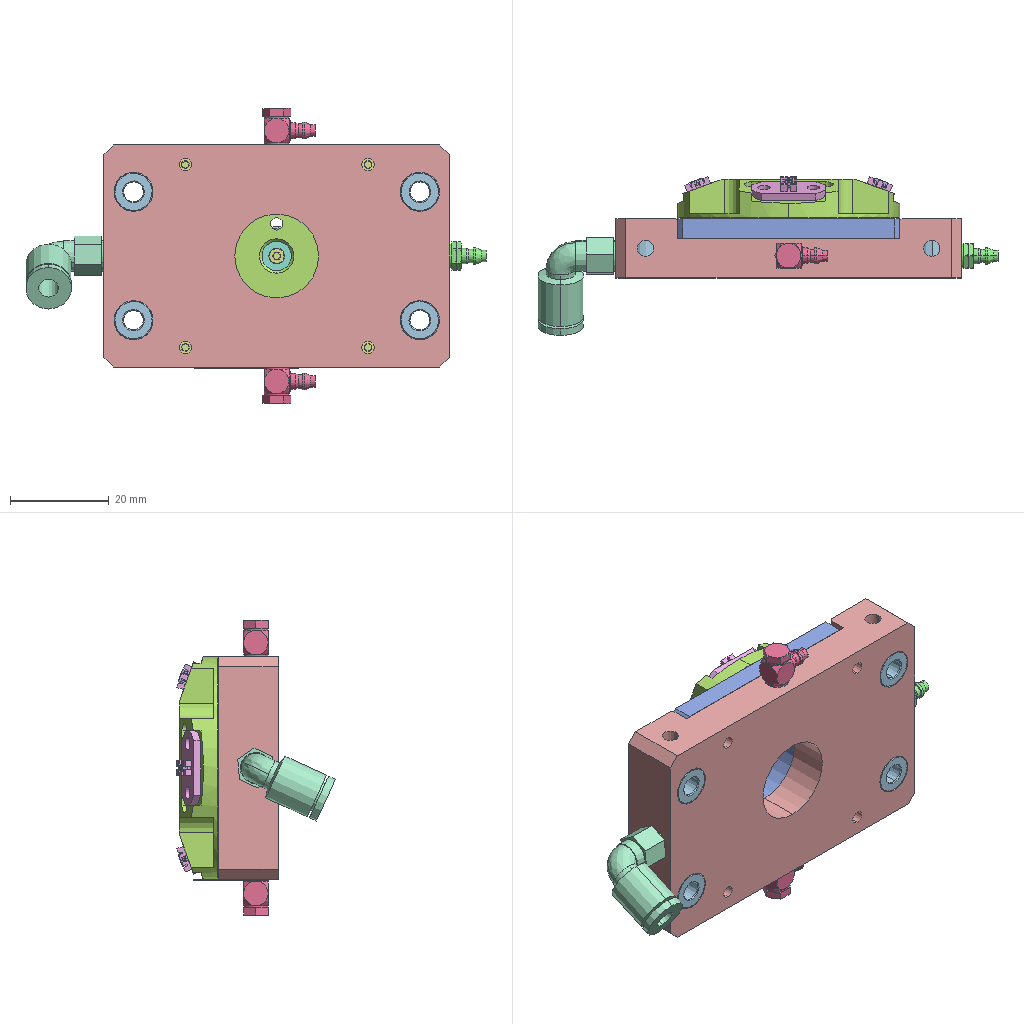Assembly | SolidWorks | 13 different items | 27 placed | box 93 x 32 x 60 mm
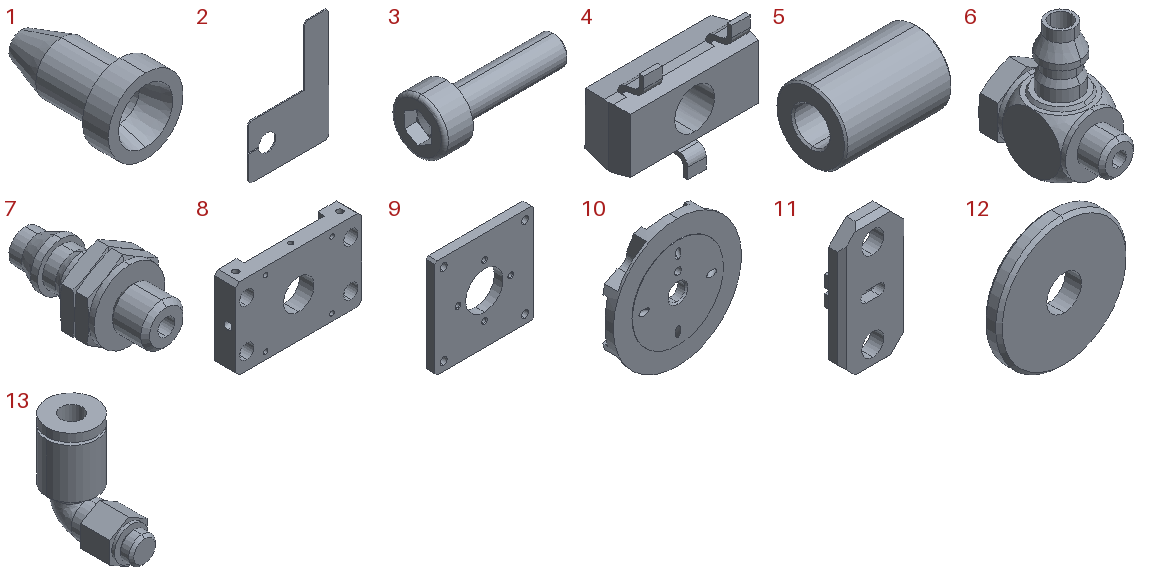Parts list (item | quantity | size | volume | features):
1 | x1 | 2.9 x 4.8 x 2.9 mm | 9.616 mm3 | features ICE 4, Chamfer 1, Extrusion 1, RevCut 1
2 | x1 | 15 x 0.2 x 21 mm | 38.09 mm3 | features ICE 3, Chamfer 1, FlatPattern 1, SMBaseFlange 1, SheetMetal 1
3 | x5 | 7.6 x 3 x 3 mm | 21.652 mm3 | features Fillet 2, RevCut 2, Boss 1, Chamfer 1, Cut 1, Extrusion 1, LPattern 1
4 | x4 | 2.908 x 1.057 x 2.408 mm | 2.992 mm3 | features ICE 6, Fillet 4, Extrusion 1, RefAxis 1
5 | x4 | 12 x 8 x 8 mm | 450.881 mm3 | features RefAxis 3, 3DProfileFeature 1, Chamfer 1, Revolution 1
6 | x2 | 5 x 9.5 x 10.687 mm | 200.167 mm3 | features BaseBody 1
7 | x1 | 5 x 10 x 5.774 mm | 89.646 mm3 | features BaseBody 1
8 | x1 | 70 x 12 x 45 mm | 24347 mm3 | features ICE 8, HoleWzd 6, 3DProfileFeature 4, Chamfer 2, CirPattern 1, Extrusion 1, MirrorPattern 1
9 | x1 | 45 x 4 x 45 mm | 6746 mm3 | features ICE 5, Chamfer 2, CirPattern 2, Cut 1, Extrusion 1, Fillet 1
10 | x1 | 45 x 8 x 45 mm | 6154 mm3 | features ICE 14, CirPattern 5, Chamfer 2, Extrusion 1, Fillet 1, HoleWzd 1
11 | x4 | 7 x 3 x 15 mm | 138.292 mm3 | features ICE 14, Chamfer 5, Extrusion 1
12 | x1 | 12 x 1.5 x 12 mm | 154.246 mm3 | features Chamfer 1, Extrusion 1
13 | x1 | 9.3 x 18.35 x 19.641 mm | 1123 mm3 | features BaseBody 1
Mates (type | each side: item.copy, entity, surface, feature):
Coincident | 8.1 face plane Cut-Extrude1 | 9.1 face plane Boss-Extrude1 | 2 times
Coincident | 8.1 face plane Boss-Extrude1 | 5.1 face plane Revolve1 | 2 times
Concentric | 8.1 face cylinder Cut-Extrude2 | 5.1 face cylinder Revolve1
Concentric | 8.1 face cylinder Cut-Extrude2 | 5.2 face cylinder Revolve1
Coincident | 8.1 face plane Boss-Extrude1 | 5.2 face plane Revolve1
Concentric | 8.1 face cylinder Cut-Extrude2 | 5.3 face cylinder Revolve1
Coincident | 8.1 face plane Boss-Extrude1 | 5.3 face plane Revolve1
Concentric | 8.1 face cylinder Cut-Extrude2 | 5.4 face cylinder Revolve1
Coincident | 8.1 face plane Boss-Extrude1 | 5.4 face plane Revolve1
Coincident | 10.1 face plane CirPattern2 | 11.1 face plane Boss-Extrude1 | 3 times
Coincident | 9.1 face plane Boss-Extrude1 | 10.1 face plane Boss-Extrude1
Concentric | 9.1 face cylinder Cut-Extrude1 | 10.1 face cylinder Boss-Extrude1
Coincident | 11.1 face plane Cut-Extrude1 | 4.1 face plane Boss-Extrude1
Concentric | 9.1 face cylinder Cut-Extrude6 | 3.1 face cylinder BaseBody
Concentric | 9.1 face cylinder CirPattern2 | 3.2 face cylinder BaseBody
Coincident | 9.1 face plane Cut-Extrude6 | 3.2 face plane BaseHead
Concentric | 9.1 face cylinder CirPattern2 | 3.3 face cylinder BaseBody
Coincident | 9.1 face plane Cut-Extrude6 | 3.3 face plane BaseHead
Concentric | 9.1 face cylinder Cut-Extrude4 | 3.4 face cylinder BaseBody
Coincident | 9.1 face plane Cut-Extrude6 | 3.4 face plane BaseHead
Coincident | 9.1 face plane Cut-Extrude6 | 3.1 face plane BaseHead
Coincident | 10.1 face plane Cut-Extrude4 | 12.1 face plane Boss-Extrude1
Concentric | 10.1 face cylinder Boss-Extrude3 | 12.1 face cylinder Boss-Extrude1
Concentric | 12.1 face cylinder Boss-Extrude1 | 3.5 face cylinder BaseBody
Coincident | 12.1 face plane Boss-Extrude1 | 3.5 face plane BaseHead
Coincident | 8.1 face plane Boss-Extrude1 | 6.1 face plane Input1
Concentric | 8.1 face cylinder CirPattern1 | 6.1 face cylinder Input1
Parallel | 8.1 face plane Boss-Extrude1 | 6.1 face plane Input1
Coincident | 8.1 face plane Boss-Extrude1 | 6.2 face plane Input1
Concentric | 8.1 face cylinder CirPattern1 | 6.2 face cylinder Input1
Parallel | 8.1 face plane Boss-Extrude1 | 6.2 face plane Input1
Coincident | 8.1 face plane Boss-Extrude1 | 9.1 face plane Boss-Extrude1
Coincident | 8.1 face plane Boss-Extrude1 | 7.1 face plane Input1
Concentric | 7.1 face cylinder Input1 | 8.1 face cylinder CirPattern1
Parallel | 8.1 face plane Boss-Extrude1 | 10.1 face plane CirPattern3
Concentric | 9.1 face cylinder Cut-Extrude2 | 1.1 face cylinder Boss-Extrude1
Coincident | 9.1 face plane Boss-Extrude1 | 1.1 face plane Boss-Extrude2
Width | 4.1 face plane Cut-Extrude2 | 4.1 face plane Cut-Extrude2 | 11.1 face plane Cut-Extrude5 | 11.1 face plane Cut-Extrude5
Concentric | 11.1 face cylinder Cut-Extrude11 | 4.1 face cylinder Cut-Extrude5
Concentric | 8.1 face cylinder M3 Tapped Hole6 | 2.1 face cylinder Cut-Extrude2
Coincident | 8.1 face plane Boss-Extrude1 | 2.1 face plane Base-Flange1
Coincident | 8.1 face plane Boss-Extrude1 | 13.1 face plane Input1
Concentric | 8.1 face cylinder M5 Tapped Hole1 | 13.1 face cylinder Input1